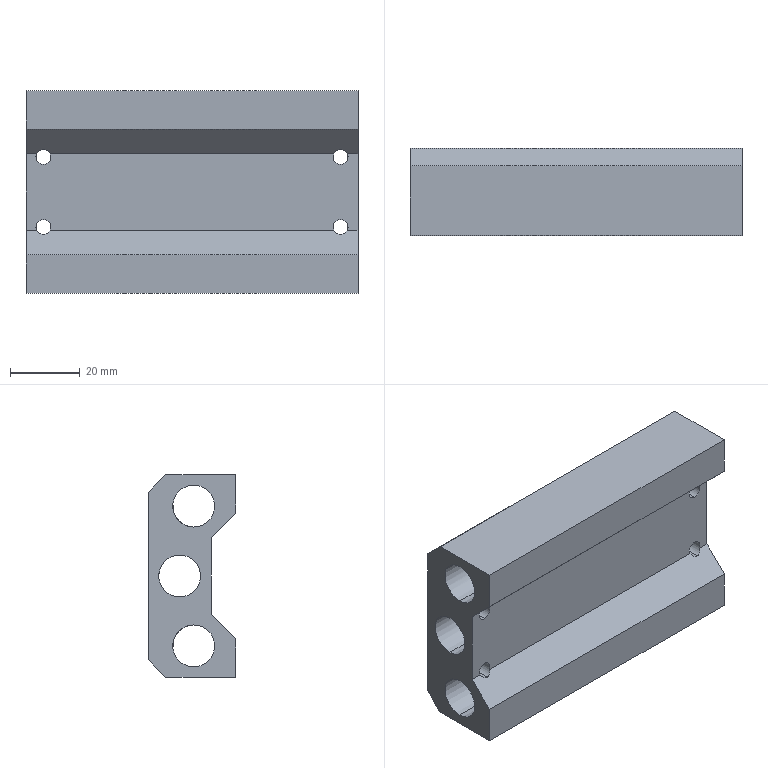Part | STEP file | 1 solid | 102 faces | box 95 x 25 x 58 mm | volume 76550 mm3 | cylinder 66 | plane 24 | cone 12 | commonest cylinder face diameters 8.4 x36 2.5 x16 4.3 x8 12 x6